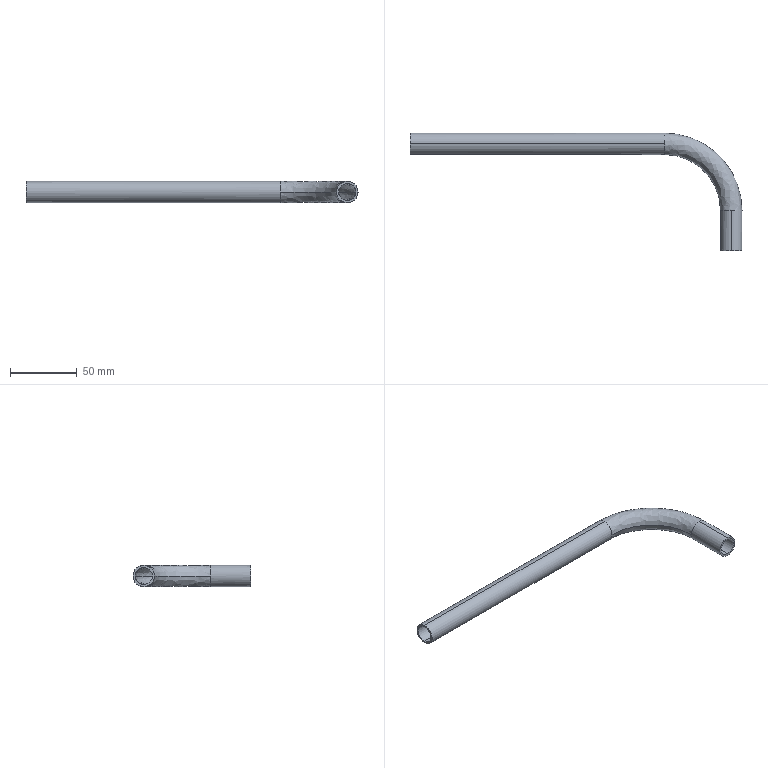Part | STEP file | copper tube 11_default_machined_ | 1 solid | 14 faces | box 248 x 88 x 16 mm | volume 20399 mm3 | cylinder 8 | spline 4 | plane 2 | commonest cylinder face diameters 13 x4 16 x4